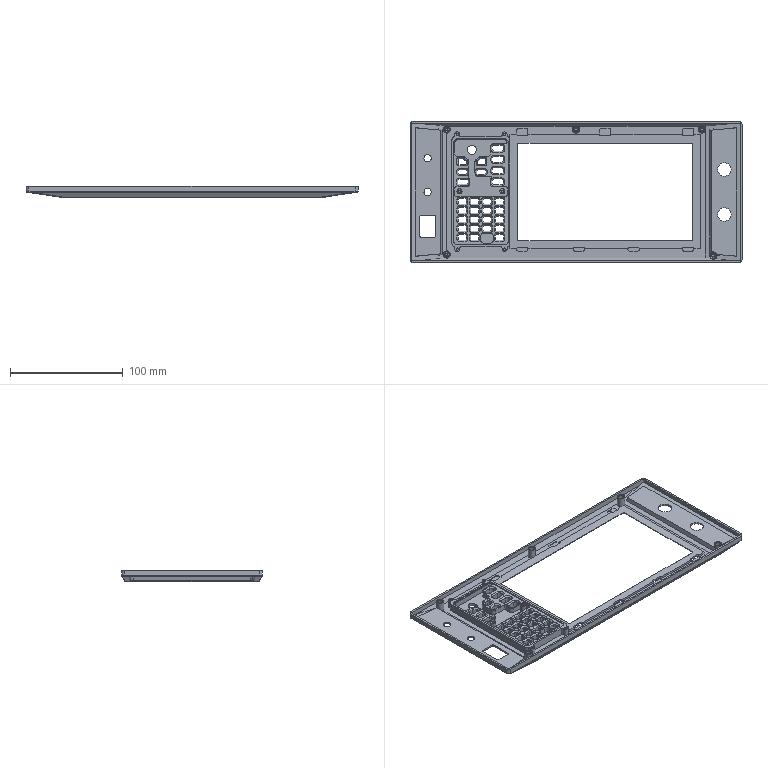NC program | NX | posted with a generic post | part box 295 x 125 x 10 mm
Lines 8754 to 10380 of 10380:
(ZLEVEL_PROFILE_1_COPY_COPY_COPY_COPY_COPY_COPY_COPY , TOOL : D4)
N17464 T04 M6
N17466 G54
N17468 G17 G0 G90 X53.178 Y-46.17 S9500 M3
N17470 G43 Z30. H4
N17472 Z-0.3
N17474 G94 G1 X53.525 Y-46.77 F1000.
N17476 G3 X53.871 Y-46.97 R0.4
N17478 G1 X55.17 F1600.
N17480 Y-45.671
N17482 G3 X54.97 Y-45.325 R0.4
N17484 G1 X54.37 Y-44.978
N17486 G0 X53.178 Y-46.17 Z-0.725
N17488 G1 X53.525 Y-46.77 F1000.
N17490 G3 X53.871 Y-46.97 R0.4
N17492 G1 X55.17 F1600.
N17494 Y-45.671
N17496 G3 X54.97 Y-45.325 R0.4
N17498 G1 X54.37 Y-44.978
N17500 G0 X53.178 Y-46.17 Z-1.15
N17502 G1 X53.525 Y-46.77 F1000.
N17504 G3 X53.871 Y-46.97 R0.4
N17506 G1 X55.17 F1600.
N17508 Y-45.671
N17510 G3 X54.97 Y-45.325 R0.4
N17512 G1 X54.37 Y-44.978
N17514 G0 X53.178 Y-46.17 Z-1.575
N17516 G1 X53.525 Y-46.77 F1000.
N17518 G3 X53.871 Y-46.97 R0.4
N17520 G1 X55.17 F1600.
N17522 Y-45.671
N17524 G3 X54.97 Y-45.325 R0.4
N17526 G1 X54.37 Y-44.978
N17528 G0 X53.178 Y-46.17 Z-2.
N17530 G1 X53.525 Y-46.77 F1000.
N17532 G3 X53.871 Y-46.97 R0.4
N17534 G1 X55.17 F1600.
N17536 Y-45.671
N17538 G3 X54.97 Y-45.325 R0.4
N17540 G1 X54.37 Y-44.978
N17542 G0 Z30.
N17544 Y47.226
N17546 Z-0.3
N17548 G1 X54.97 Y47.572 F1000.
N17550 G3 X55.17 Y47.919 R0.4
N17552 G1 Y48.795 F1600.
N17554 X54.411 Y49.234
N17556 G3 X54.011 Y49.234 R0.4
N17558 G1 X53.411 Y48.887
N17560 G0 Z30.
N17562 X54.37 Y45.958
N17564 Z-0.725
N17566 G1 X54.97 Y46.305 F1000.
N17568 G3 X55.17 Y46.651 R0.4
N17570 G1 Y47.95 F1600.
N17572 X53.871
N17574 G3 X53.525 Y47.75 R0.4
N17576 G1 X53.178 Y47.15
N17578 G0 X54.37 Y45.958 Z-1.15
N17580 G1 X54.97 Y46.305 F1000.
N17582 G3 X55.17 Y46.651 R0.4
N17584 G1 Y47.95 F1600.
N17586 X53.871
N17588 G3 X53.525 Y47.75 R0.4
N17590 G1 X53.178 Y47.15
N17592 G0 X54.37 Y45.958 Z-1.575
N17594 G1 X54.97 Y46.305 F1000.
N17596 G3 X55.17 Y46.651 R0.4
N17598 G1 Y47.95 F1600.
N17600 X53.871
N17602 G3 X53.525 Y47.75 R0.4
N17604 G1 X53.178 Y47.15
N17606 G0 X54.37 Y45.958 Z-2.
N17608 G1 X54.97 Y46.305 F1000.
N17610 G3 X55.17 Y46.651 R0.4
N17612 G1 Y47.95 F1600.
N17614 X53.871
N17616 G3 X53.525 Y47.75 R0.4
N17618 G1 X53.178 Y47.15
N17620 G0 Z30.
N17622 X44.363 Y54.111
N17624 Z-0.3
N17626 G1 Y54.804 F1000.
N17628 G3 X44.163 Y55.15 R0.4
N17630 G1 X43.672 Y55.434 F1600.
N17632 X43.105
N17634 G3 X42.758 Y55.234 R0.4
N17636 G1 X42.412 Y54.634
N17638 G0 Z30.
N17640 X-94.282
N17642 Z-0.3
N17644 G1 X-94.628 Y55.234 F1000.
N17646 G3 X-94.975 Y55.434 R0.4
N17648 G1 X-95.542 F1600.
N17650 X-96.033 Y55.15
N17652 G3 X-96.233 Y54.804 R0.4
N17654 G1 Y54.111
N17656 G0 Z30.
N17658 X-105.281 Y48.887
N17660 Z-0.3
N17662 G1 X-105.881 Y49.233 F1000.
N17664 G3 X-106.281 Y49.233 R0.4
N17666 G1 X-107.04 Y48.795 F1600.
N17668 Y47.919
N17670 G3 X-106.84 Y47.573 R0.4
N17672 G1 X-106.24 Y47.226
N17674 G0 X-105.048 Y47.15 Z-0.725
N17676 G1 X-105.395 Y47.75 F1000.
N17678 G3 X-105.741 Y47.95 R0.4
N17680 G1 X-107.04 F1600.
N17682 Y46.651
N17684 G3 X-106.84 Y46.305 R0.4
N17686 G1 X-106.24 Y45.958
N17688 G0 X-105.048 Y47.15 Z-1.15
N17690 G1 X-105.395 Y47.75 F1000.
N17692 G3 X-105.741 Y47.95 R0.4
N17694 G1 X-107.04 F1600.
N17696 Y46.651
N17698 G3 X-106.84 Y46.305 R0.4
N17700 G1 X-106.24 Y45.958
N17702 G0 X-105.048 Y47.15 Z-1.575
N17704 G1 X-105.395 Y47.75 F1000.
N17706 G3 X-105.741 Y47.95 R0.4
N17708 G1 X-107.04 F1600.
N17710 Y46.651
N17712 G3 X-106.84 Y46.305 R0.4
N17714 G1 X-106.24 Y45.958
N17716 G0 X-105.048 Y47.15 Z-2.
N17718 G1 X-105.395 Y47.75 F1000.
N17720 G3 X-105.741 Y47.95 R0.4
N17722 G1 X-107.04 F1600.
N17724 Y46.651
N17726 G3 X-106.84 Y46.305 R0.4
N17728 G1 X-106.24 Y45.958
N17730 G0 Z30.
N17732 Y-44.978
N17734 Z-0.3
N17736 G1 X-106.84 Y-45.325 F1000.
N17738 G3 X-107.04 Y-45.671 R0.4
N17740 G1 Y-46.97 F1600.
N17742 X-105.741
N17744 G3 X-105.395 Y-46.77 R0.4
N17746 G1 X-105.048 Y-46.17
N17748 G0 X-106.24 Y-44.978 Z-0.725
N17750 G1 X-106.84 Y-45.325 F1000.
N17752 G3 X-107.04 Y-45.671 R0.4
N17754 G1 Y-46.97 F1600.
N17756 X-105.741
N17758 G3 X-105.395 Y-46.77 R0.4
N17760 G1 X-105.048 Y-46.17
N17762 G0 X-106.24 Y-44.978 Z-1.15
N17764 G1 X-106.84 Y-45.325 F1000.
N17766 G3 X-107.04 Y-45.671 R0.4
N17768 G1 Y-46.97 F1600.
N17770 X-105.741
N17772 G3 X-105.395 Y-46.77 R0.4
N17774 G1 X-105.048 Y-46.17
N17776 G0 X-106.24 Y-44.978 Z-1.575
N17778 G1 X-106.84 Y-45.325 F1000.
N17780 G3 X-107.04 Y-45.671 R0.4
N17782 G1 Y-46.97 F1600.
N17784 X-105.741
N17786 G3 X-105.395 Y-46.77 R0.4
N17788 G1 X-105.048 Y-46.17
N17790 G0 X-106.24 Y-44.978 Z-2.
N17792 G1 X-106.84 Y-45.325 F1000.
N17794 G3 X-107.04 Y-45.671 R0.4
N17796 G1 Y-46.97 F1600.
N17798 X-105.741
N17800 G3 X-105.395 Y-46.77 R0.4
N17802 G1 X-105.048 Y-46.17
N17804 G0 Z30.
N17806 M5
(ZLEVEL_PROFILE_1_COPY_COPY_COPY_COPY_COPY_COPY_COPY_COPY , TOOL : D2)
N17808 T02 M6
N17810 G54
N17812 G17 G0 G90 X54.525 Y-47.57 S9500 M3
N17814 G43 Z30. H2
N17816 Z-0.2
N17818 G94 G1 X54.698 Y-47.87 F1000.
N17820 G3 X54.871 Y-47.97 R0.2
N17822 G1 X56.17 F1200.
N17824 Y-46.671
N17826 G3 X56.07 Y-46.498 R0.2
N17828 G1 X55.77 Y-46.325
N17830 G0 X54.525 Y-47.57 Z-0.3
N17832 G1 X54.698 Y-47.87 F1000.
N17834 G3 X54.871 Y-47.97 R0.2
N17836 G1 X56.17 F1200.
N17838 Y-46.671
N17840 G3 X56.07 Y-46.498 R0.2
N17842 G1 X55.77 Y-46.325
N17844 G0 X54.525 Y-47.57 Z-0.5
N17846 G1 X54.698 Y-47.87 F1000.
N17848 G3 X54.871 Y-47.97 R0.2
N17850 G1 X56.17 F1200.
N17852 Y-46.671
N17854 G3 X56.07 Y-46.498 R0.2
N17856 G1 X55.77 Y-46.325
N17858 G0 X54.525 Y-47.57 Z-0.7
N17860 G1 X54.698 Y-47.87 F1000.
N17862 G3 X54.871 Y-47.97 R0.2
N17864 G1 X56.17 F1200.
N17866 Y-46.671
N17868 G3 X56.07 Y-46.498 R0.2
N17870 G1 X55.77 Y-46.325
N17872 G0 X54.525 Y-47.57 Z-0.9
N17874 G1 X54.698 Y-47.87 F1000.
N17876 G3 X54.871 Y-47.97 R0.2
N17878 G1 X56.17 F1200.
N17880 Y-46.671
N17882 G3 X56.07 Y-46.498 R0.2
N17884 G1 X55.77 Y-46.325
N17886 G0 X54.525 Y-47.57 Z-1.1
N17888 G1 X54.698 Y-47.87 F1000.
N17890 G3 X54.871 Y-47.97 R0.2
N17892 G1 X56.17 F1200.
N17894 Y-46.671
N17896 G3 X56.07 Y-46.498 R0.2
N17898 G1 X55.77 Y-46.325
N17900 G0 X54.525 Y-47.57 Z-1.3
N17902 G1 X54.698 Y-47.87 F1000.
N17904 G3 X54.871 Y-47.97 R0.2
N17906 G1 X56.17 F1200.
N17908 Y-46.671
N17910 G3 X56.07 Y-46.498 R0.2
N17912 G1 X55.77 Y-46.325
N17914 G0 X54.525 Y-47.57 Z-1.475
N17916 G1 X54.698 Y-47.87 F1000.
N17918 G3 X54.871 Y-47.97 R0.2
N17920 G1 X56.17 F1200.
N17922 Y-46.671
N17924 G3 X56.07 Y-46.498 R0.2
N17926 G1 X55.77 Y-46.325
N17928 G0 X54.525 Y-47.57 Z-1.65
N17930 G1 X54.698 Y-47.87 F1000.
N17932 G3 X54.871 Y-47.97 R0.2
N17934 G1 X56.17 F1200.
N17936 Y-46.671
N17938 G3 X56.07 Y-46.498 R0.2
N17940 G1 X55.77 Y-46.325
N17942 G0 X54.525 Y-47.57 Z-1.825
N17944 G1 X54.698 Y-47.87 F1000.
N17946 G3 X54.871 Y-47.97 R0.2
N17948 G1 X56.17 F1200.
N17950 Y-46.671
N17952 G3 X56.07 Y-46.498 R0.2
N17954 G1 X55.77 Y-46.325
N17956 G0 X54.525 Y-47.57 Z-2.
N17958 G1 X54.698 Y-47.87 F1000.
N17960 G3 X54.871 Y-47.97 R0.2
N17962 G1 X56.17 F1200.
N17964 Y-46.671
N17966 G3 X56.07 Y-46.498 R0.2
N17968 G1 X55.77 Y-46.325
N17970 G0 Z30.
N17972 Y48.15
N17974 Z-0.2
N17976 G1 X56.07 Y48.323 F1000.
N17978 G3 X56.17 Y48.496 R0.2
N17980 G1 Y49.373 F1200.
N17982 X55.411 Y49.811
N17984 G3 X55.211 Y49.811 R0.2
N17986 G1 X54.911 Y49.638
N17988 G0 X55.77 Y48.15 Z-0.3
N17990 G1 X56.07 Y48.323 F1000.
N17992 G3 X56.17 Y48.496 R0.2
N17994 G1 Y49.373 F1200.
N17996 X55.411 Y49.811
N17998 G3 X55.211 Y49.811 R0.2
N18000 G1 X54.911 Y49.638
N18002 G0 Z30.
N18004 X55.77 Y47.305
N18006 Z-0.5
N18008 G1 X56.07 Y47.478 F1000.
N18010 G3 X56.17 Y47.651 R0.2
N18012 G1 Y48.95 F1200.
N18014 X54.871
N18016 G3 X54.698 Y48.85 R0.2
N18018 G1 X54.525 Y48.55
N18020 G0 X55.77 Y47.305 Z-0.7
N18022 G1 X56.07 Y47.478 F1000.
N18024 G3 X56.17 Y47.651 R0.2
N18026 G1 Y48.95 F1200.
N18028 X54.871
N18030 G3 X54.698 Y48.85 R0.2
N18032 G1 X54.525 Y48.55
N18034 G0 X55.77 Y47.305 Z-0.9
N18036 G1 X56.07 Y47.478 F1000.
N18038 G3 X56.17 Y47.651 R0.2
N18040 G1 Y48.95 F1200.
N18042 X54.871
N18044 G3 X54.698 Y48.85 R0.2
N18046 G1 X54.525 Y48.55
N18048 G0 X55.77 Y47.305 Z-1.1
N18050 G1 X56.07 Y47.478 F1000.
N18052 G3 X56.17 Y47.651 R0.2
N18054 G1 Y48.95 F1200.
N18056 X54.871
N18058 G3 X54.698 Y48.85 R0.2
N18060 G1 X54.525 Y48.55
N18062 G0 X55.77 Y47.305 Z-1.3
N18064 G1 X56.07 Y47.478 F1000.
N18066 G3 X56.17 Y47.651 R0.2
N18068 G1 Y48.95 F1200.
N18070 X54.871
N18072 G3 X54.698 Y48.85 R0.2
N18074 G1 X54.525 Y48.55
N18076 G0 X55.77 Y47.305 Z-1.475
N18078 G1 X56.07 Y47.478 F1000.
N18080 G3 X56.17 Y47.651 R0.2
N18082 G1 Y48.95 F1200.
N18084 X54.871
N18086 G3 X54.698 Y48.85 R0.2
N18088 G1 X54.525 Y48.55
N18090 G0 X55.77 Y47.305 Z-1.65
N18092 G1 X56.07 Y47.478 F1000.
N18094 G3 X56.17 Y47.651 R0.2
N18096 G1 Y48.95 F1200.
N18098 X54.871
N18100 G3 X54.698 Y48.85 R0.2
N18102 G1 X54.525 Y48.55
N18104 G0 X55.77 Y47.305 Z-1.825
N18106 G1 X56.07 Y47.478 F1000.
N18108 G3 X56.17 Y47.651 R0.2
N18110 G1 Y48.95 F1200.
N18112 X54.871
N18114 G3 X54.698 Y48.85 R0.2
N18116 G1 X54.525 Y48.55
N18118 G0 X55.77 Y47.305 Z-2.
N18120 G1 X56.07 Y47.478 F1000.
N18122 G3 X56.17 Y47.651 R0.2
N18124 G1 Y48.95 F1200.
N18126 X54.871
N18128 G3 X54.698 Y48.85 R0.2
N18130 G1 X54.525 Y48.55
N18132 G0 Z30.
N18134 X44.531 Y55.631
N18136 Z-0.2
N18138 G1 Y55.977 F1000.
N18140 G3 X44.431 Y56.15 R0.2
N18142 G1 X43.94 Y56.434 F1200.
N18144 X43.373
N18146 G3 X43.2 Y56.334 R0.2
N18148 G1 X43.026 Y56.034
N18150 G0 X44.531 Y55.631 Z-0.3
N18152 G1 Y55.977 F1000.
N18154 G3 X44.431 Y56.15 R0.2
N18156 G1 X43.94 Y56.434 F1200.
N18158 X43.373
N18160 G3 X43.2 Y56.334 R0.2
N18162 G1 X43.026 Y56.034
N18164 G0 Z30.
N18166 X-94.896
N18168 Z-0.2
N18170 G1 X-95.07 Y56.334 F1000.
N18172 G3 X-95.243 Y56.434 R0.2
N18174 G1 X-95.81 F1200.
N18176 X-96.301 Y56.15
N18178 G3 X-96.401 Y55.977 R0.2
N18180 G1 Y55.631
N18182 G0 X-94.896 Y56.034 Z-0.3
N18184 G1 X-95.07 Y56.334 F1000.
N18186 G3 X-95.243 Y56.434 R0.2
N18188 G1 X-95.81 F1200.
N18190 X-96.301 Y56.15
N18192 G3 X-96.401 Y55.977 R0.2
N18194 G1 Y55.631
N18196 G0 Z30.
N18198 X-106.781 Y49.638
N18200 Z-0.2
N18202 G1 X-107.081 Y49.811 F1000.
N18204 G3 X-107.281 Y49.811 R0.2
N18206 G1 X-108.04 Y49.373 F1200.
N18208 Y48.496
N18210 G3 X-107.94 Y48.323 R0.2
N18212 G1 X-107.64 Y48.15
N18214 G0 X-106.781 Y49.638 Z-0.3
N18216 G1 X-107.081 Y49.811 F1000.
N18218 G3 X-107.281 Y49.811 R0.2
N18220 G1 X-108.04 Y49.373 F1200.
N18222 Y48.496
N18224 G3 X-107.94 Y48.323 R0.2
N18226 G1 X-107.64 Y48.15
N18228 G0 X-106.395 Y48.55 Z-0.5
N18230 G1 X-106.568 Y48.85 F1000.
N18232 G3 X-106.741 Y48.95 R0.2
N18234 G1 X-108.04 F1200.
N18236 Y47.651
N18238 G3 X-107.94 Y47.478 R0.2
N18240 G1 X-107.64 Y47.305
N18242 G0 X-106.395 Y48.55 Z-0.7
N18244 G1 X-106.568 Y48.85 F1000.
N18246 G3 X-106.741 Y48.95 R0.2
N18248 G1 X-108.04 F1200.
N18250 Y47.651
N18252 G3 X-107.94 Y47.478 R0.2
N18254 G1 X-107.64 Y47.305
N18256 G0 X-106.395 Y48.55 Z-0.9
N18258 G1 X-106.568 Y48.85 F1000.
N18260 G3 X-106.741 Y48.95 R0.2
N18262 G1 X-108.04 F1200.
N18264 Y47.651
N18266 G3 X-107.94 Y47.478 R0.2
N18268 G1 X-107.64 Y47.305
N18270 G0 X-106.395 Y48.55 Z-1.1
N18272 G1 X-106.568 Y48.85 F1000.
N18274 G3 X-106.741 Y48.95 R0.2
N18276 G1 X-108.04 F1200.
N18278 Y47.651
N18280 G3 X-107.94 Y47.478 R0.2
N18282 G1 X-107.64 Y47.305
N18284 G0 X-106.395 Y48.55 Z-1.3
N18286 G1 X-106.568 Y48.85 F1000.
N18288 G3 X-106.741 Y48.95 R0.2
N18290 G1 X-108.04 F1200.
N18292 Y47.651
N18294 G3 X-107.94 Y47.478 R0.2
N18296 G1 X-107.64 Y47.305
N18298 G0 X-106.395 Y48.55 Z-1.475
N18300 G1 X-106.568 Y48.85 F1000.
N18302 G3 X-106.741 Y48.95 R0.2
N18304 G1 X-108.04 F1200.
N18306 Y47.651
N18308 G3 X-107.94 Y47.478 R0.2
N18310 G1 X-107.64 Y47.305
N18312 G0 X-106.395 Y48.55 Z-1.65
N18314 G1 X-106.568 Y48.85 F1000.
N18316 G3 X-106.741 Y48.95 R0.2
N18318 G1 X-108.04 F1200.
N18320 Y47.651
N18322 G3 X-107.94 Y47.478 R0.2
N18324 G1 X-107.64 Y47.305
N18326 G0 X-106.395 Y48.55 Z-1.825
N18328 G1 X-106.568 Y48.85 F1000.
N18330 G3 X-106.741 Y48.95 R0.2
N18332 G1 X-108.04 F1200.
N18334 Y47.651
N18336 G3 X-107.94 Y47.478 R0.2
N18338 G1 X-107.64 Y47.305
N18340 G0 X-106.395 Y48.55 Z-2.
N18342 G1 X-106.568 Y48.85 F1000.
N18344 G3 X-106.741 Y48.95 R0.2
N18346 G1 X-108.04 F1200.
N18348 Y47.651
N18350 G3 X-107.94 Y47.478 R0.2
N18352 G1 X-107.64 Y47.305
N18354 G0 Z30.
N18356 Y-46.325
N18358 Z-0.2
N18360 G1 X-107.94 Y-46.498 F1000.
N18362 G3 X-108.04 Y-46.671 R0.2
N18364 G1 Y-47.97 F1200.
N18366 X-106.741
N18368 G3 X-106.568 Y-47.87 R0.2
N18370 G1 X-106.395 Y-47.57
N18372 G0 X-107.64 Y-46.325 Z-0.3
N18374 G1 X-107.94 Y-46.498 F1000.
N18376 G3 X-108.04 Y-46.671 R0.2
N18378 G1 Y-47.97 F1200.
N18380 X-106.741
N18382 G3 X-106.568 Y-47.87 R0.2
N18384 G1 X-106.395 Y-47.57
N18386 G0 X-107.64 Y-46.325 Z-0.5
N18388 G1 X-107.94 Y-46.498 F1000.
N18390 G3 X-108.04 Y-46.671 R0.2
N18392 G1 Y-47.97 F1200.
N18394 X-106.741
N18396 G3 X-106.568 Y-47.87 R0.2
N18398 G1 X-106.395 Y-47.57
N18400 G0 X-107.64 Y-46.325 Z-0.7
N18402 G1 X-107.94 Y-46.498 F1000.
N18404 G3 X-108.04 Y-46.671 R0.2
N18406 G1 Y-47.97 F1200.
N18408 X-106.741
N18410 G3 X-106.568 Y-47.87 R0.2
N18412 G1 X-106.395 Y-47.57
N18414 G0 X-107.64 Y-46.325 Z-0.9
N18416 G1 X-107.94 Y-46.498 F1000.
N18418 G3 X-108.04 Y-46.671 R0.2
N18420 G1 Y-47.97 F1200.
N18422 X-106.741
N18424 G3 X-106.568 Y-47.87 R0.2
N18426 G1 X-106.395 Y-47.57
N18428 G0 X-107.64 Y-46.325 Z-1.1
N18430 G1 X-107.94 Y-46.498 F1000.
N18432 G3 X-108.04 Y-46.671 R0.2
N18434 G1 Y-47.97 F1200.
N18436 X-106.741
N18438 G3 X-106.568 Y-47.87 R0.2
N18440 G1 X-106.395 Y-47.57
N18442 G0 X-107.64 Y-46.325 Z-1.3
N18444 G1 X-107.94 Y-46.498 F1000.
N18446 G3 X-108.04 Y-46.671 R0.2
N18448 G1 Y-47.97 F1200.
N18450 X-106.741
N18452 G3 X-106.568 Y-47.87 R0.2
N18454 G1 X-106.395 Y-47.57
N18456 G0 X-107.64 Y-46.325 Z-1.475
N18458 G1 X-107.94 Y-46.498 F1000.
N18460 G3 X-108.04 Y-46.671 R0.2
N18462 G1 Y-47.97 F1200.
N18464 X-106.741
N18466 G3 X-106.568 Y-47.87 R0.2
N18468 G1 X-106.395 Y-47.57
N18470 G0 X-107.64 Y-46.325 Z-1.65
N18472 G1 X-107.94 Y-46.498 F1000.
N18474 G3 X-108.04 Y-46.671 R0.2
N18476 G1 X-108.039 Y-47.97 F1200.
N18478 X-106.741
N18480 G3 X-106.568 Y-47.87 R0.2
N18482 G1 X-106.395 Y-47.57
N18484 G0 X-107.64 Y-46.325 Z-1.825
N18486 G1 X-107.94 Y-46.498 F1000.
N18488 G3 X-108.04 Y-46.671 R0.2
N18490 G1 X-108.039 Y-47.97 F1200.
N18492 X-106.741
N18494 G3 X-106.568 Y-47.87 R0.2
N18496 G1 X-106.395 Y-47.57
N18498 G0 X-107.64 Y-46.325 Z-2.
N18500 G1 X-107.94 Y-46.498 F1000.
N18502 G3 X-108.04 Y-46.671 R0.2
N18504 G1 X-108.039 Y-47.97 F1200.
N18506 X-106.741
N18508 G3 X-106.568 Y-47.87 R0.2
N18510 G1 X-106.395 Y-47.57
N18512 G0 Z30.
N18514 M5
(ZLEVEL_PROFILE_1_COPY_COPY_COPY_COPY_COPY , TOOL : D2R0.5)
N18516 T05 M6
N18518 G54
N18520 G17 G0 G90 X51.029 Y45.352 S9500 M3
N18522 G43 Z30. H5
N18524 Z-0.532
N18526 G94 G1 Z-2.032 F1000.
N18528 X50.843 Y45.674
N18530 G3 X50.67 Y45.774 R0.2
N18532 G1 X-102.54 F3000.
N18534 G3 X-105.864 Y42.45 R3.324
N18536 G1 Y-42.47
N18538 G3 X-102.54 Y-45.794 R3.324
N18540 G1 X50.67
N18542 G3 X53.994 Y-42.47 R3.324
N18544 G1 Y42.45
N18546 G3 X50.67 Y45.774 R3.324
N18548 G1 Y45.679 Z-2.063
N18550 G2 X53.899 Y42.45 R3.229
N18552 G1 Y-42.47
N18554 G2 X50.67 Y-45.699 R3.229
N18556 G1 X-102.54
N18558 G2 X-105.769 Y-42.47 R3.229
N18560 G1 Y42.45
N18562 G2 X-102.54 Y45.679 R3.229
N18564 G1 X50.67
N18566 Y45.584 Z-2.095
N18568 X-102.54
N18570 G3 X-105.674 Y42.45 R3.134
N18572 G1 Y-42.47
N18574 G3 X-102.54 Y-45.604 R3.134
N18576 G1 X50.67
N18578 G3 X53.804 Y-42.47 R3.134
N18580 G1 Y42.45
N18582 G3 X50.67 Y45.584 R3.134
N18584 G1 Y45.489 Z-2.126
N18586 G2 X53.709 Y42.45 R3.039
N18588 G1 Y-42.47
N18590 G2 X50.67 Y-45.509 R3.039
N18592 G1 X-102.54
N18594 G2 X-105.579 Y-42.47 R3.039
N18596 G1 Y42.45
N18598 G2 X-102.54 Y45.489 R3.039
N18600 G1 X50.67
N18602 Y45.395 Z-2.158
N18604 X-102.54
N18606 G3 X-105.485 Y42.45 R2.945
N18608 G1 Y-42.47
N18610 G3 X-102.54 Y-45.415 R2.945
N18612 G1 X50.67
N18614 G3 X53.615 Y-42.47 R2.945
N18616 G1 Y42.45
N18618 G3 X50.67 Y45.395 R2.945
N18620 G1 Y45.3 Z-2.19
N18622 G2 X53.52 Y42.45 R2.85
N18624 G1 Y-42.47
N18626 G2 X50.67 Y-45.32 R2.85
N18628 G1 X-102.54
N18630 G2 X-105.39 Y-42.47 R2.85
N18632 G1 Y42.45
N18634 G2 X-102.54 Y45.3 R2.85
N18636 G1 X50.67
N18638 Y45.205 Z-2.221
N18640 X-102.54
N18642 G3 X-105.295 Y42.45 R2.755
N18644 G1 Y-42.47
N18646 G3 X-102.54 Y-45.225 R2.755
N18648 G1 X50.67
N18650 G3 X53.425 Y-42.47 R2.755
N18652 G1 Y42.45
N18654 G3 X50.67 Y45.205 R2.755
N18656 G1 Y45.11 Z-2.253
N18658 G2 X53.33 Y42.45 R2.66
N18660 G1 Y-42.47
N18662 G2 X50.67 Y-45.13 R2.66
N18664 G1 X-102.54
N18666 G2 X-105.2 Y-42.47 R2.66
N18668 G1 Y42.45
N18670 G2 X-102.54 Y45.11 R2.66
N18672 G1 X50.67
N18674 Y45.015 Z-2.285
N18676 X-102.54
N18678 G3 X-105.105 Y42.45 R2.565
N18680 G1 Y-42.47
N18682 G3 X-102.54 Y-45.035 R2.565
N18684 G1 X50.67
N18686 G3 X53.235 Y-42.47 R2.565
N18688 G1 Y42.45
N18690 G3 X50.67 Y45.015 R2.565
N18692 G1 Y44.92 Z-2.316
N18694 G2 X53.14 Y42.45 R2.47
N18696 G1 Y-42.47
N18698 G2 X50.67 Y-44.94 R2.47
N18700 G1 X-102.54
N18702 G2 X-105.01 Y-42.47 R2.47
N18704 G1 Y42.45
N18706 G2 X-102.54 Y44.92 R2.47
N18708 G1 X50.67
N18710 Y44.825 Z-2.348
N18712 X-102.54
N18714 G3 X-104.915 Y42.45 R2.375
N18716 G1 Y-42.47
N18718 G3 X-102.54 Y-44.845 R2.375
N18720 G1 X50.67
N18722 G3 X53.045 Y-42.47 R2.375
N18724 G1 Y42.45
N18726 G3 X50.67 Y44.825 R2.375
N18728 G1 Y44.73 Z-2.379
N18730 G2 X52.95 Y42.45 R2.28
N18732 G1 Y-42.47
N18734 G2 X50.67 Y-44.75 R2.28
N18736 G1 X-102.54
N18738 G2 X-104.82 Y-42.47 R2.28
N18740 G1 Y42.45
N18742 G2 X-102.54 Y44.73 R2.28
N18744 G1 X50.67
N18746 Y44.636 Z-2.411
N18748 X-102.54
N18750 G3 X-104.726 Y42.45 R2.186
N18752 G1 Y-42.47
N18754 G3 X-102.54 Y-44.656 R2.186
N18756 G1 X50.67
N18758 G3 X52.856 Y-42.47 R2.186
N18760 G1 Y42.45
N18762 G3 X50.67 Y44.636 R2.186
N18764 G1 Y44.541 Z-2.443
N18766 G2 X52.761 Y42.45 R2.091
N18768 G1 Y-42.47
N18770 G2 X50.67 Y-44.561 R2.091
N18772 G1 X-102.54
N18774 G2 X-104.631 Y-42.47 R2.091
N18776 G1 Y42.45
N18778 G2 X-102.54 Y44.541 R2.091
N18780 G1 X50.67
N18782 Y44.446 Z-2.474
N18784 X-102.54
N18786 G3 X-104.536 Y42.45 R1.996
N18788 G1 Y-42.47
N18790 G3 X-102.54 Y-44.466 R1.996
N18792 G1 X50.67
N18794 G3 X52.666 Y-42.47 R1.996
N18796 G1 Y42.45
N18798 G3 X50.67 Y44.446 R1.996
N18800 G1 Y44.351 Z-2.506
N18802 G2 X52.571 Y42.45 R1.901
N18804 G1 Y-42.47
N18806 G2 X50.67 Y-44.371 R1.901
N18808 G1 X-102.54
N18810 G2 X-104.441 Y-42.47 R1.901
N18812 G1 Y42.45
N18814 G2 X-102.54 Y44.351 R1.901
N18816 G1 X50.67
N18818 Y44.256 Z-2.538
N18820 X-102.54
N18822 G3 X-104.346 Y42.45 R1.806
N18824 G1 Y-42.47
N18826 G3 X-102.54 Y-44.276 R1.806
N18828 G1 X50.67
N18830 G3 X52.476 Y-42.47 R1.806
N18832 G1 Y42.45
N18834 G3 X50.67 Y44.256 R1.806
N18836 G1 Y44.161 Z-2.569
N18838 G2 X52.381 Y42.45 R1.711
N18840 G1 Y-42.47
N18842 G2 X50.67 Y-44.181 R1.711
N18844 G1 X-102.54
N18846 G2 X-104.251 Y-42.47 R1.711
N18848 G1 Y42.45
N18850 G2 X-102.54 Y44.161 R1.711
N18852 G1 X50.67
N18854 Y44.066 Z-2.601
N18856 X-102.54
N18858 G3 X-104.156 Y42.45 R1.616
N18860 G1 Y-42.47
N18862 G3 X-102.54 Y-44.086 R1.616
N18864 G1 X50.67
N18866 G3 X52.286 Y-42.47 R1.616
N18868 G1 Y42.45
N18870 G3 X50.67 Y44.066 R1.616
N18872 G1 Y43.971 Z-2.632
N18874 G2 X52.191 Y42.45 R1.521
N18876 G1 Y-42.47
N18878 G2 X50.67 Y-43.991 R1.521
N18880 G1 X-102.54
N18882 G2 X-104.061 Y-42.47 R1.521
N18884 G1 Y42.45
N18886 G2 X-102.54 Y43.971 R1.521
N18888 G1 X50.67
N18890 Y43.877 Z-2.664
N18892 X-102.54
N18894 G3 X-103.967 Y42.45 R1.427
N18896 G1 Y-42.47
N18898 G3 X-102.54 Y-43.897 R1.427
N18900 G1 X50.67
N18902 G3 X52.097 Y-42.47 R1.427
N18904 G1 Y42.45
N18906 G3 X50.67 Y43.877 R1.427
N18908 G1 Y43.782 Z-2.696
N18910 G2 X52.002 Y42.45 R1.332
N18912 G1 Y-42.47
N18914 G2 X50.67 Y-43.802 R1.332
N18916 G1 X-102.54
N18918 G2 X-103.872 Y-42.47 R1.332
N18920 G1 Y42.45
N18922 G2 X-102.54 Y43.782 R1.332
N18924 G1 X50.67
N18926 Y43.687 Z-2.727
N18928 X-102.54
N18930 G3 X-103.777 Y42.45 R1.237
N18932 G1 Y-42.47
N18934 G3 X-102.54 Y-43.707 R1.237
N18936 G1 X50.67
N18938 G3 X51.907 Y-42.47 R1.237
N18940 G1 Y42.45
N18942 G3 X50.67 Y43.687 R1.237
N18944 G1 Y43.592 Z-2.759
N18946 G2 X51.812 Y42.45 R1.142
N18948 G1 Y-42.47
N18950 G2 X50.67 Y-43.612 R1.142
N18952 G1 X-102.54
N18954 G2 X-103.682 Y-42.47 R1.142
N18956 G1 Y42.45
N18958 G2 X-102.54 Y43.592 R1.142
N18960 G1 X50.67
N18962 Y43.497 Z-2.791
N18964 X-102.54
N18966 G3 X-103.587 Y42.45 R1.047
N18968 G1 Y-42.47
N18970 G3 X-102.54 Y-43.517 R1.047
N18972 G1 X50.67
N18974 G3 X51.717 Y-42.47 R1.047
N18976 G1 Y42.45
N18978 G3 X50.67 Y43.497 R1.047
N18980 G1 Y43.402 Z-2.822
N18982 G2 X51.622 Y42.45 R0.952
N18984 G1 Y-42.47
N18986 G2 X50.67 Y-43.422 R0.952
N18988 G1 X-102.54
N18990 G2 X-103.492 Y-42.47 R0.952
N18992 G1 Y42.45
N18994 G2 X-102.54 Y43.402 R0.952
N18996 G1 X50.67
N18998 Y43.307 Z-2.854
N19000 X-102.54
N19002 G3 X-103.397 Y42.45 R0.857
N19004 G1 Y-42.47
N19006 G3 X-102.54 Y-43.327 R0.857
N19008 G1 X50.67
N19010 G3 X51.527 Y-42.47 R0.857
N19012 G1 Y42.45
N19014 G3 X50.67 Y43.307 R0.857
N19016 G1 Y43.213 Z-2.885
N19018 G2 X51.433 Y42.45 R0.763
N19020 G1 Y-42.47
N19022 G2 X50.67 Y-43.233 R0.763
N19024 G1 X-102.54
N19026 G2 X-103.303 Y-42.47 R0.763
N19028 G1 Y42.45
N19030 G2 X-102.54 Y43.213 R0.763
N19032 G1 X50.67
N19034 Y43.118 Z-2.917
N19036 X-102.54
N19038 G3 X-103.208 Y42.45 R0.668
N19040 G1 Y-42.47
N19042 G3 X-102.54 Y-43.138 R0.668
N19044 G1 X50.67
N19046 G3 X51.338 Y-42.47 R0.668
N19048 G1 Y42.45
N19050 G3 X50.67 Y43.118 R0.668
N19052 G1 Y43.023 Z-2.949
N19054 G2 X51.243 Y42.45 R0.573
N19056 G1 Y-42.47
N19058 G2 X50.67 Y-43.043 R0.573
N19060 G1 X-102.54
N19062 G2 X-103.113 Y-42.47 R0.573
N19064 G1 Y42.45
N19066 G2 X-102.54 Y43.023 R0.573
N19068 G1 X50.67
N19070 Y42.928 Z-2.98
N19072 X-102.54
N19074 G3 X-103.018 Y42.45 R0.478
N19076 G1 Y-42.47
N19078 G3 X-102.54 Y-42.948 R0.478
N19080 G1 X50.67
N19082 G3 X51.148 Y-42.47 R0.478
N19084 G1 Y42.45
N19086 G3 X50.67 Y42.928 R0.478
N19088 G1 Y42.833 Z-3.012
N19090 G2 X51.053 Y42.45 R0.383
N19092 G1 Y-42.47
N19094 G2 X50.67 Y-42.853 R0.383
N19096 G1 X-102.54
N19098 G2 X-102.923 Y-42.47 R0.383
N19100 G1 Y42.45
N19102 G2 X-102.54 Y42.833 R0.383
N19104 G1 X50.67
N19106 X50.669 Y42.785 Z-3.028
N19108 X50.668 Y42.738 Z-3.044
N19110 X-102.534
N19112 G3 X-102.828 Y42.444 R0.294
N19114 G1 Y-42.464
N19116 G3 X-102.534 Y-42.758 R0.294
N19118 G1 X50.664
N19120 G3 X50.958 Y-42.464 R0.294
N19122 G1 Y42.444
N19124 G3 X50.668 Y42.738 R0.294
N19126 G1 X50.666 Y42.689 Z-3.059
N19128 X50.664 Y42.642 Z-3.075
N19130 G2 X50.863 Y42.434 R0.208
N19132 G1 Y-42.455
N19134 G2 X50.655 Y-42.663 R0.208
N19136 G1 X-102.525
N19138 G2 X-102.733 Y-42.455 R0.208
N19140 G1 Y42.435
N19142 G2 X-102.525 Y42.643 R0.208
N19144 G1 X50.664 Y42.642
N19146 X50.663 Y42.594 Z-3.091
N19148 X50.661 Y42.547 Z-3.107
N19150 X-102.528
N19152 X-102.588 Y42.542
N19154 X-102.631 Y42.498
N19156 X-102.637 Y42.439
N19158 Y-42.442
N19160 X-102.547 Y-42.565
N19162 X50.658 Y-42.567
N19164 X50.718 Y-42.562
N19166 X50.761 Y-42.518
N19168 X50.767 Y-42.459
N19170 Y42.438
N19172 X50.762 Y42.497
N19174 X50.72 Y42.54
N19176 X50.661 Y42.547
N19178 X50.658 Y42.498 Z-3.123
N19180 X50.655 Y42.45 Z-3.138
N19182 Y-42.47
N19184 X-102.447 Y-42.472
N19186 X-102.54 Y-42.442
N19188 X-102.525 Y42.45
N19190 X50.655
N19192 G2 X50.555 Y42.277 R0.2
N19194 G1 X50.163 Y42.05
N19196 Z-1.638
N19198 G0 Z30.
N19200 X50.084 Y41.957
N19202 Z-1.67
N19204 G1 Z-3.17 F1000.
N19206 X50.477 Y42.184
N19208 G3 X50.577 Y42.357 R0.2
N19210 G1 X-102.447 Y42.358 F3000.
N19212 X-102.448 Y-42.375
N19214 X50.577 Y-42.378
N19216 Y42.357
N19218 G3 X50.404 Y42.257 R0.2
N19220 G1 X50.177 Y41.865
N19222 Z-1.67
N19224 G0 Z30.
N19226 M5
(ZLEVEL_PROFILE_COPY_1 , TOOL : D6A45)
N19228 T07 M6
N19230 G54
N19232 G17 G0 G90 X72.81 Y30.012 S9500 M3
N19234 G43 Z30. H7
N19236 Z0.5
N19238 G94 G1 Z-1. F1000.
N19240 X73.02 Y30.391
N19242 G3 X72.5 Y30.691 R0.6
N19244 G1 X66.5
N19246 G3 X65.259 Y29.45 R1.241
N19248 G1 Y28.45
N19250 G3 X66.5 Y27.209 R1.241
N19252 G1 X72.5
N19254 G3 X73.741 Y28.45 R1.241
N19256 G1 Y29.45
N19258 G3 X72.5 Y30.691 R1.241
N19260 X71.98 Y30.391 R0.6
N19262 G1 X71.807 Y30.091
N19264 Z0.5
N19266 G0 Z30.
N19268 X98.859 Y25.901
N19270 Z0.5
N19272 G1 Z-1.
N19274 X98.559 Y25.728
N19276 G3 X98.259 Y25.209 R0.6
N19278 G1 X103.741
N19280 Y28.691
N19282 X101.077
N19284 G2 X98.259 Y26.628 R12.259
N19286 G1 Y25.209
N19288 G3 X98.778 Y25.509 R0.6
N19290 G1 X98.951 Y25.809
N19292 Z0.5
N19294 G0 Z30.
N19296 X81.859 Y25.901
N19298 Z0.5
N19300 G1 Z-1.
N19302 X81.559 Y25.728
N19304 G3 X81.259 Y25.209 R0.6
N19306 G1 X86.741
N19308 Y26.628
N19310 G2 X83.923 Y28.691 R12.259
N19312 G1 X81.259
N19314 Y25.209
N19316 G3 X81.778 Y25.509 R0.6
N19318 G1 X81.951 Y25.809
N19320 Z0.5
N19322 G0 Z30.
N19324 X72.81 Y20.012
N19326 Z0.5
N19328 G1 Z-1.
N19330 X73.02 Y20.391
N19332 G3 X72.5 Y20.691 R0.6
N19334 G1 X66.5
N19336 G3 X65.259 Y19.45 R1.241
N19338 G1 Y18.45
N19340 G3 X66.5 Y17.209 R1.241
N19342 G1 X72.5
N19344 G3 X73.741 Y18.45 R1.241
N19346 G1 Y19.45
N19348 G3 X72.5 Y20.691 R1.241
N19350 X71.98 Y20.391 R0.6
N19352 G1 X71.807 Y20.091
N19354 Z0.5
N19356 G0 Z30.
N19358 X103.31 Y18.262
N19360 Z0.5
N19362 G1 Z-1.
N19364 X103.52 Y18.641
N19366 G3 X103. Y18.941 R0.6
N19368 G1 X98.
N19370 G3 X97.759 Y18.7 R0.241
N19372 G1 Y16.7
N19374 G3 X98. Y16.459 R0.241
N19376 G1 X103.
N19378 G3 X104.241 Y17.7 R1.241
N19380 X103. Y18.941 R1.241
N19382 X102.48 Y18.641 R0.6
N19384 G1 X102.307 Y18.341
N19386 Z0.5
N19388 G0 Z30.
N19390 X86.561
N19392 Z0.5
N19394 G1 Z-1.
N19396 X86.7 Y18.422
N19398 G3 X87. Y18.941 R0.6
N19400 G1 X82.
N19402 G3 X80.759 Y17.7 R1.241
N19404 X82. Y16.459 R1.241
N19406 G1 X87.
N19408 G3 X87.241 Y16.7 R0.241
N19410 G1 Y18.7
N19412 G3 X87. Y18.941 R0.241
N19414 X86.48 Y18.641 R0.6
N19416 G1 X86.307 Y18.341
N19418 Z0.5
N19420 G0 Z30.
N19422 X103.561 Y9.591
N19424 Z0.5
N19426 G1 Z-1.
N19428 X103.7 Y9.672
N19430 G3 X104. Y10.191 R0.6
N19432 G1 X97.
N19434 G3 X96.759 Y9.95 R0.241
N19436 G1 Y7.95
N19438 G3 X97. Y7.709 R0.241
N19440 G1 X104.
N19442 G3 X104.241 Y7.95 R0.241
N19444 G1 Y9.95
N19446 G3 X104. Y10.191 R0.241
N19448 X103.48 Y9.891 R0.6
N19450 G1 X103.307 Y9.591
N19452 Z0.5
N19454 G0 Z30.
N19456 X72.81 Y10.012
N19458 Z0.5
N19460 G1 Z-1.
N19462 X73.02 Y10.391
N19464 G3 X72.5 Y10.691 R0.6
N19466 G1 X66.5
N19468 G3 X65.259 Y9.45 R1.241
N19470 G1 Y8.45
N19472 G3 X66.5 Y7.209 R1.241
N19474 G1 X72.5
N19476 G3 X73.741 Y8.45 R1.241
N19478 G1 Y9.45
N19480 G3 X72.5 Y10.691 R1.241
N19482 X71.98 Y10.391 R0.6
N19484 G1 X71.807 Y10.091
N19486 Z0.5
N19488 G0 Z30.
N19490 X103.019 Y-7.129
N19492 Z0.5
N19494 G1 Z-1.
N19496 X103.114 Y-7.066
N19498 G3 X103.382 Y-6.529 R0.6
N19500 G1 X98.618
N19502 G3 X98.402 Y-6.662 R0.241
N19504 G1 X98.284 Y-6.898
N19506 X98.255 Y-6.948
N19508 X98.259 Y-7.006
N19510 Y-9.534
N19512 X98.255 Y-9.592
N19514 X98.284 Y-9.642
N19516 X98.402 Y-9.878
N19518 G3 X98.618 Y-10.011 R0.241
N19520 G1 X103.382
N19522 G3 X103.598 Y-9.878 R0.241
N19524 G1 X103.716 Y-9.642
N19526 X103.745 Y-9.592
N19528 X103.741 Y-9.534
N19530 Y-7.006
N19532 X103.745 Y-6.948
N19534 X103.716 Y-6.898
N19536 X103.598 Y-6.662
N19538 G3 X103.382 Y-6.529 R0.241
N19540 X102.862 Y-6.829 R0.6
N19542 G1 X102.689 Y-7.129
N19544 Z0.5
N19546 G0 Z30.
N19548 X87.981 Y-9.411
N19550 Z0.5
N19552 G1 Z-1.
N19554 X87.886 Y-9.474
N19556 G3 X87.618 Y-10.011 R0.6
N19558 G1 X92.382
N19560 G3 X92.598 Y-9.878 R0.241
N19562 G1 X92.716 Y-9.642
N19564 X92.745 Y-9.592
N19566 X92.741 Y-9.534
N19568 Y-7.006
N19570 X92.745 Y-6.948
N19572 X92.716 Y-6.898
N19574 X92.598 Y-6.662
N19576 G3 X92.382 Y-6.529 R0.241
N19578 G1 X87.618
N19580 G3 X87.402 Y-6.662 R0.241
N19582 G1 X87.284 Y-6.898
N19584 X87.255 Y-6.948
N19586 X87.259 Y-7.006
N19588 Y-9.534
N19590 X87.255 Y-9.592
N19592 X87.284 Y-9.642
N19594 X87.402 Y-9.878
N19596 G3 X87.618 Y-10.011 R0.241
N19598 X88.138 Y-9.711 R0.6
N19600 G1 X88.311 Y-9.411
N19602 Z0.5
N19604 G0 Z30.
N19606 X76.981
N19608 Z0.5
N19610 G1 Z-1.
N19612 X76.886 Y-9.474
N19614 G3 X76.618 Y-10.011 R0.6
N19616 G1 X81.382
N19618 G3 X81.598 Y-9.878 R0.241
N19620 G1 X81.716 Y-9.642
N19622 X81.745 Y-9.592
N19624 X81.741 Y-9.534
N19626 Y-7.006
N19628 X81.745 Y-6.948
N19630 X81.716 Y-6.898
N19632 X81.598 Y-6.662
N19634 G3 X81.382 Y-6.529 R0.241
N19636 G1 X76.618
N19638 G3 X76.402 Y-6.662 R0.241
N19640 G1 X76.284 Y-6.898
N19642 X76.255 Y-6.948
N19644 X76.259 Y-7.006
N19646 Y-9.534
N19648 X76.255 Y-9.592
N19650 X76.284 Y-9.642
N19652 X76.402 Y-9.878
N19654 G3 X76.618 Y-10.011 R0.241
N19656 X77.138 Y-9.711 R0.6
N19658 G1 X77.311 Y-9.411
N19660 Z0.5
N19662 G0 Z30.
N19664 X65.981
N19666 Z0.5
N19668 G1 Z-1.
N19670 X65.886 Y-9.474
N19672 G3 X65.618 Y-10.011 R0.6
N19674 G1 X70.382
N19676 G3 X70.598 Y-9.878 R0.241
N19678 G1 X70.716 Y-9.642
N19680 X70.745 Y-9.592
N19682 X70.741 Y-9.534
N19684 Y-7.006
N19686 X70.745 Y-6.948
N19688 X70.716 Y-6.898
N19690 X70.598 Y-6.662
N19692 G3 X70.382 Y-6.529 R0.241
N19694 G1 X65.618
N19696 G3 X65.402 Y-6.662 R0.241
N19698 G1 X65.284 Y-6.898
N19700 X65.255 Y-6.948
N19702 X65.259 Y-7.006
N19704 Y-9.534
N19706 X65.255 Y-9.592
N19708 X65.284 Y-9.642
N19710 X65.402 Y-9.878
N19712 G3 X65.618 Y-10.011 R0.241
N19714 X66.138 Y-9.711 R0.6
N19716 G1 X66.311 Y-9.411
N19718 Z0.5
N19720 G0 Z30.
N19722 X98.981 Y-17.411
N19724 Z0.5
N19726 G1 Z-1.
N19728 X98.886 Y-17.474
N19730 G3 X98.618 Y-18.011 R0.6
N19732 G1 X103.382
N19734 G3 X103.598 Y-17.878 R0.241
N19736 G1 X103.716 Y-17.642
N19738 X103.745 Y-17.592
N19740 X103.741 Y-17.534
N19742 Y-15.006
N19744 X103.745 Y-14.948
N19746 X103.716 Y-14.898
N19748 X103.598 Y-14.662
N19750 G3 X103.382 Y-14.529 R0.241
N19752 G1 X98.618
N19754 G3 X98.402 Y-14.662 R0.241
N19756 G1 X98.284 Y-14.898
N19758 X98.255 Y-14.948
N19760 X98.259 Y-15.006
N19762 Y-17.534
N19764 X98.255 Y-17.592
N19766 X98.284 Y-17.642
N19768 X98.402 Y-17.878
N19770 G3 X98.618 Y-18.011 R0.241
N19772 X99.138 Y-17.711 R0.6
N19774 G1 X99.311 Y-17.411
N19776 Z0.5
N19778 G0 Z30.
N19780 X87.981
N19782 Z0.5
N19784 G1 Z-1.
N19786 X87.886 Y-17.474
N19788 G3 X87.618 Y-18.011 R0.6
N19790 G1 X92.382
N19792 G3 X92.598 Y-17.878 R0.241
N19794 G1 X92.716 Y-17.642
N19796 X92.745 Y-17.592
N19798 X92.741 Y-17.534
N19800 Y-15.006
N19802 X92.745 Y-14.948
N19804 X92.716 Y-14.898
N19806 X92.598 Y-14.662
N19808 G3 X92.382 Y-14.529 R0.241
N19810 G1 X87.618
N19812 G3 X87.402 Y-14.662 R0.241
N19814 G1 X87.284 Y-14.898
N19816 X87.255 Y-14.948
N19818 X87.259 Y-15.006
N19820 Y-17.534
N19822 X87.255 Y-17.592
N19824 X87.284 Y-17.642
N19826 X87.402 Y-17.878
N19828 G3 X87.618 Y-18.011 R0.241
N19830 X88.138 Y-17.711 R0.6
N19832 G1 X88.311 Y-17.411
N19834 Z0.5
N19836 G0 Z30.
N19838 X76.981
N19840 Z0.5
N19842 G1 Z-1.
N19844 X76.886 Y-17.474
N19846 G3 X76.618 Y-18.011 R0.6
N19848 G1 X81.382
N19850 G3 X81.598 Y-17.878 R0.241
N19852 G1 X81.716 Y-17.642
N19854 X81.745 Y-17.592
N19856 X81.741 Y-17.534
N19858 Y-15.006
N19860 X81.745 Y-14.948
N19862 X81.716 Y-14.898
N19864 X81.598 Y-14.662
N19866 G3 X81.382 Y-14.529 R0.241
N19868 G1 X76.618
N19870 G3 X76.402 Y-14.662 R0.241
N19872 G1 X76.284 Y-14.898
N19874 X76.255 Y-14.948
N19876 X76.259 Y-15.006
N19878 Y-17.534
N19880 X76.255 Y-17.592
N19882 X76.284 Y-17.642
N19884 X76.402 Y-17.878
N19886 G3 X76.618 Y-18.011 R0.241
N19888 X77.138 Y-17.711 R0.6
N19890 G1 X77.311 Y-17.411
N19892 Z0.5
N19894 G0 Z30.
N19896 X65.981
N19898 Z0.5
N19900 G1 Z-1.
N19902 X65.886 Y-17.474
N19904 G3 X65.618 Y-18.011 R0.6
N19906 G1 X70.382
N19908 G3 X70.598 Y-17.878 R0.241
N19910 G1 X70.716 Y-17.642
N19912 X70.745 Y-17.592
N19914 X70.741 Y-17.534
N19916 Y-15.006
N19918 X70.745 Y-14.948
N19920 X70.716 Y-14.898
N19922 X70.598 Y-14.662
N19924 G3 X70.382 Y-14.529 R0.241
N19926 G1 X65.618
N19928 G3 X65.402 Y-14.662 R0.241
N19930 G1 X65.284 Y-14.898
N19932 X65.255 Y-14.948
N19934 X65.259 Y-15.006
N19936 Y-17.534
N19938 X65.255 Y-17.592
N19940 X65.284 Y-17.642
N19942 X65.402 Y-17.878
N19944 G3 X65.618 Y-18.011 R0.241
N19946 X66.138 Y-17.711 R0.6
N19948 G1 X66.311 Y-17.411
N19950 Z0.5
N19952 G0 Z30.
N19954 X98.981 Y-25.411
N19956 Z0.5
N19958 G1 Z-1.
N19960 X98.886 Y-25.474
N19962 G3 X98.618 Y-26.011 R0.6
N19964 G1 X103.382
N19966 G3 X103.598 Y-25.878 R0.241
N19968 G1 X103.716 Y-25.642
N19970 X103.745 Y-25.592
N19972 X103.741 Y-25.534
N19974 Y-23.006
N19976 X103.745 Y-22.948
N19978 X103.716 Y-22.898
N19980 X103.598 Y-22.662
N19982 G3 X103.382 Y-22.529 R0.241
N19984 G1 X98.618
N19986 G3 X98.402 Y-22.662 R0.241
N19988 G1 X98.284 Y-22.898
N19990 X98.255 Y-22.948
N19992 X98.259 Y-23.006
N19994 Y-25.534
N19996 X98.255 Y-25.592
N19998 X98.284 Y-25.642
N20000 X98.402 Y-25.878
N20002 G3 X98.618 Y-26.011 R0.241
N20004 X99.138 Y-25.711 R0.6
N20006 G1 X99.311 Y-25.411
N20008 Z0.5
N20010 G0 Z30.
N20012 X87.981
N20014 Z0.5
N20016 G1 Z-1.
N20018 X87.886 Y-25.474
N20020 G3 X87.618 Y-26.011 R0.6
N20022 G1 X92.382
N20024 G3 X92.598 Y-25.878 R0.241
N20026 G1 X92.716 Y-25.642
N20028 X92.745 Y-25.592
N20030 X92.741 Y-25.534
N20032 Y-23.006
N20034 X92.745 Y-22.948
N20036 X92.716 Y-22.898
N20038 X92.598 Y-22.662
N20040 G3 X92.382 Y-22.529 R0.241
N20042 G1 X87.618
N20044 G3 X87.402 Y-22.662 R0.241
N20046 G1 X87.284 Y-22.898
N20048 X87.255 Y-22.948
N20050 X87.259 Y-23.006
N20052 Y-25.534
N20054 X87.255 Y-25.592
N20056 X87.284 Y-25.642
N20058 X87.402 Y-25.878
N20060 G3 X87.618 Y-26.011 R0.241
N20062 X88.138 Y-25.711 R0.6
N20064 G1 X88.311 Y-25.411
N20066 Z0.5
N20068 G0 Z30.
N20070 X76.981
N20072 Z0.5
N20074 G1 Z-1.
N20076 X76.886 Y-25.474
N20078 G3 X76.618 Y-26.011 R0.6
N20080 G1 X81.382
N20082 G3 X81.598 Y-25.878 R0.241
N20084 G1 X81.716 Y-25.642
N20086 X81.745 Y-25.592
N20088 X81.741 Y-25.534
N20090 Y-23.006
N20092 X81.745 Y-22.948
N20094 X81.716 Y-22.898
N20096 X81.598 Y-22.662
N20098 G3 X81.382 Y-22.529 R0.241
N20100 G1 X76.618
N20102 G3 X76.402 Y-22.662 R0.241
N20104 G1 X76.284 Y-22.898
N20106 X76.255 Y-22.948
N20108 X76.259 Y-23.006
N20110 Y-25.534
N20112 X76.255 Y-25.592
N20114 X76.284 Y-25.642
N20116 X76.402 Y-25.878
N20118 G3 X76.618 Y-26.011 R0.241
N20120 X77.138 Y-25.711 R0.6
N20122 G1 X77.311 Y-25.411
N20124 Z0.5
N20126 G0 Z30.
N20128 X65.981
N20130 Z0.5
N20132 G1 Z-1.
N20134 X65.886 Y-25.474
N20136 G3 X65.618 Y-26.011 R0.6
N20138 G1 X70.382
N20140 G3 X70.598 Y-25.878 R0.241
N20142 G1 X70.716 Y-25.642
N20144 X70.745 Y-25.592
N20146 X70.741 Y-25.534
N20148 Y-23.006
N20150 X70.745 Y-22.948
N20152 X70.716 Y-22.898
N20154 X70.598 Y-22.662
N20156 G3 X70.382 Y-22.529 R0.241
N20158 G1 X65.618
N20160 G3 X65.402 Y-22.662 R0.241
N20162 G1 X65.284 Y-22.898
N20164 X65.255 Y-22.948
N20166 X65.259 Y-23.006
N20168 Y-25.534
N20170 X65.255 Y-25.592
N20172 X65.284 Y-25.642
N20174 X65.402 Y-25.878
N20176 G3 X65.618 Y-26.011 R0.241
N20178 X66.138 Y-25.711 R0.6
N20180 G1 X66.311 Y-25.411
N20182 Z0.5
N20184 G0 Z30.
N20186 X98.981 Y-33.411
N20188 Z0.5
N20190 G1 Z-1.
N20192 X98.886 Y-33.474
N20194 G3 X98.618 Y-34.011 R0.6
N20196 G1 X103.382
N20198 G3 X103.598 Y-33.878 R0.241
N20200 G1 X103.716 Y-33.642
N20202 X103.745 Y-33.592
N20204 X103.741 Y-33.534
N20206 Y-31.006
N20208 X103.745 Y-30.948
N20210 X103.716 Y-30.898
N20212 X103.598 Y-30.662
N20214 G3 X103.382 Y-30.529 R0.241
N20216 G1 X98.618
N20218 G3 X98.402 Y-30.662 R0.241
N20220 G1 X98.284 Y-30.898
N20222 X98.255 Y-30.948
N20224 X98.259 Y-31.006
N20226 Y-33.534
N20228 X98.255 Y-33.592
N20230 X98.284 Y-33.642
N20232 X98.402 Y-33.878
N20234 G3 X98.618 Y-34.011 R0.241
N20236 X99.138 Y-33.711 R0.6
N20238 G1 X99.311 Y-33.411
N20240 Z0.5
N20242 G0 Z30.
N20244 X87.981
N20246 Z0.5
N20248 G1 Z-1.
N20250 X87.886 Y-33.474
N20252 G3 X87.618 Y-34.011 R0.6
N20254 G1 X92.382
N20256 G3 X92.598 Y-33.878 R0.241
N20258 G1 X92.716 Y-33.642
N20260 X92.745 Y-33.592
N20262 X92.741 Y-33.534
N20264 Y-31.006
N20266 X92.745 Y-30.948
N20268 X92.716 Y-30.898
N20270 X92.598 Y-30.662
N20272 G3 X92.382 Y-30.529 R0.241
N20274 G1 X87.618
N20276 G3 X87.402 Y-30.662 R0.241
N20278 G1 X87.284 Y-30.898
N20280 X87.255 Y-30.948
N20282 X87.259 Y-31.006
N20284 Y-33.534
N20286 X87.255 Y-33.592
N20288 X87.284 Y-33.642
N20290 X87.402 Y-33.878
N20292 G3 X87.618 Y-34.011 R0.241
N20294 X88.138 Y-33.711 R0.6
N20296 G1 X88.311 Y-33.411
N20298 Z0.5
N20300 G0 Z30.
N20302 X76.981
N20304 Z0.5
N20306 G1 Z-1.
N20308 X76.886 Y-33.474
N20310 G3 X76.618 Y-34.011 R0.6
N20312 G1 X81.382
N20314 G3 X81.598 Y-33.878 R0.241
N20316 G1 X81.716 Y-33.642
N20318 X81.745 Y-33.592
N20320 X81.741 Y-33.534
N20322 Y-31.006
N20324 X81.745 Y-30.948
N20326 X81.716 Y-30.898
N20328 X81.598 Y-30.662
N20330 G3 X81.382 Y-30.529 R0.241
N20332 G1 X76.618
N20334 G3 X76.402 Y-30.662 R0.241
N20336 G1 X76.284 Y-30.898
N20338 X76.255 Y-30.948
N20340 X76.259 Y-31.006
N20342 Y-33.534
N20344 X76.255 Y-33.592
N20346 X76.284 Y-33.642
N20348 X76.402 Y-33.878
N20350 G3 X76.618 Y-34.011 R0.241
N20352 X77.138 Y-33.711 R0.6
N20354 G1 X77.311 Y-33.411
N20356 Z0.5
N20358 G0 Z30.
N20360 X65.981
N20362 Z0.5
N20364 G1 Z-1.
N20366 X65.886 Y-33.474
N20368 G3 X65.618 Y-34.011 R0.6
N20370 G1 X70.382
N20372 G3 X70.598 Y-33.878 R0.241
N20374 G1 X70.716 Y-33.642
N20376 X70.745 Y-33.592
N20378 X70.741 Y-33.534
N20380 Y-31.006
N20382 X70.745 Y-30.948
N20384 X70.716 Y-30.898
N20386 X70.598 Y-30.662
N20388 G3 X70.382 Y-30.529 R0.241
N20390 G1 X65.618
N20392 G3 X65.402 Y-30.662 R0.241
N20394 G1 X65.284 Y-30.898
N20396 X65.255 Y-30.948
N20398 X65.259 Y-31.006
N20400 Y-33.534
N20402 X65.255 Y-33.592
N20404 X65.284 Y-33.642
N20406 X65.402 Y-33.878
N20408 G3 X65.618 Y-34.011 R0.241
N20410 X66.138 Y-33.711 R0.6
N20412 G1 X66.311 Y-33.411
N20414 Z0.5
N20416 G0 Z30.
N20418 X72.81 Y40.012
N20420 Z0.5
N20422 G1 Z-1.
N20424 X73.02 Y40.391
N20426 G3 X72.5 Y40.691 R0.6
N20428 G1 X66.5
N20430 G3 X65.259 Y39.45 R1.241
N20432 G1 Y38.45
N20434 G3 X66.5 Y37.209 R1.241
N20436 G1 X72.5
N20438 G3 X73.741 Y38.45 R1.241
N20440 G1 Y39.45
N20442 G3 X72.5 Y40.691 R1.241
N20444 X71.98 Y40.391 R0.6
N20446 G1 X71.807 Y40.091
N20448 Z0.5
N20450 G0 Z30.
N20452 X98.981 Y-41.411
N20454 Z0.5
N20456 G1 Z-1.
N20458 X98.886 Y-41.474
N20460 G3 X98.618 Y-42.011 R0.6
N20462 G1 X103.382
N20464 G3 X103.598 Y-41.878 R0.241
N20466 G1 X103.716 Y-41.642
N20468 X103.745 Y-41.592
N20470 X103.741 Y-41.534
N20472 Y-39.006
N20474 X103.745 Y-38.948
N20476 X103.716 Y-38.898
N20478 X103.598 Y-38.662
N20480 G3 X103.382 Y-38.529 R0.241
N20482 G1 X98.618
N20484 G3 X98.402 Y-38.662 R0.241
N20486 G1 X98.284 Y-38.898
N20488 X98.255 Y-38.948
N20490 X98.259 Y-39.006
N20492 Y-41.534
N20494 X98.255 Y-41.592
N20496 X98.284 Y-41.642
N20498 X98.402 Y-41.878
N20500 G3 X98.618 Y-42.011 R0.241
N20502 X99.138 Y-41.711 R0.6
N20504 G1 X99.311 Y-41.411
N20506 Z0.5
N20508 G0 Z30.
N20510 X87.981
N20512 Z0.5
N20514 G1 Z-1.
N20516 X87.886 Y-41.474
N20518 G3 X87.618 Y-42.011 R0.6
N20520 G1 X92.382
N20522 G3 X92.598 Y-41.878 R0.241
N20524 G1 X92.716 Y-41.642
N20526 X92.745 Y-41.592
N20528 X92.741 Y-41.534
N20530 Y-39.006
N20532 X92.745 Y-38.948
N20534 X92.716 Y-38.898
N20536 X92.598 Y-38.662
N20538 G3 X92.382 Y-38.529 R0.241
N20540 G1 X87.618
N20542 G3 X87.402 Y-38.662 R0.241
N20544 G1 X87.284 Y-38.898
N20546 X87.255 Y-38.948
N20548 X87.259 Y-39.006
N20550 Y-41.534
N20552 X87.255 Y-41.592
N20554 X87.284 Y-41.642
N20556 X87.402 Y-41.878
N20558 G3 X87.618 Y-42.011 R0.241
N20560 X88.138 Y-41.711 R0.6
N20562 G1 X88.311 Y-41.411
N20564 Z0.5
N20566 G0 Z30.
N20568 X65.981
N20570 Z0.5
N20572 G1 Z-1.
N20574 X65.886 Y-41.474
N20576 G3 X65.618 Y-42.011 R0.6
N20578 G1 X70.382
N20580 G3 X70.598 Y-41.878 R0.241
N20582 G1 X70.716 Y-41.642
N20584 X70.745 Y-41.592
N20586 X70.741 Y-41.534
N20588 Y-39.006
N20590 X70.745 Y-38.948
N20592 X70.716 Y-38.898
N20594 X70.598 Y-38.662
N20596 G3 X70.382 Y-38.529 R0.241
N20598 G1 X65.618
N20600 G3 X65.402 Y-38.662 R0.241
N20602 G1 X65.284 Y-38.898
N20604 X65.255 Y-38.948
N20606 X65.259 Y-39.006
N20608 Y-41.534
N20610 X65.255 Y-41.592
N20612 X65.284 Y-41.642
N20614 X65.402 Y-41.878
N20616 G3 X65.618 Y-42.011 R0.241
N20618 X66.138 Y-41.711 R0.6
N20620 G1 X66.311 Y-41.411
N20622 Z0.5
N20624 G0 Z30.
N20626 X-107.481 Y-47.343
N20628 Z0.5
N20630 G1 Z-1.
N20632 X-107.74 Y-47.492
N20634 G3 X-108.04 Y-48.011 R0.6
N20636 G1 X56.17
N20638 X56.196 Y-48.015
N20640 X56.215 Y-47.996
N20642 X56.211 Y-47.97
N20644 Y49.289
N20646 X56.17 Y49.291
N20648 X-108.04
N20650 X-108.081 Y49.289
N20652 Y-47.97
N20654 X-108.085 Y-47.996
N20656 X-108.066 Y-48.015
N20658 X-108.04 Y-48.011
N20660 G3 X-107.52 Y-47.711 R0.6
N20662 G1 X-107.347 Y-47.411
N20664 Z0.5
N20666 G0 Z30.
N20668 X93.264 Y39.769
N20670 Z0.5
N20672 G1 Z-1.
N20674 X93.02 Y40.191
N20676 G3 X92.5 Y40.491 R0.6
N20678 X89.459 Y37.45 R3.041
N20680 X92.5 Y40.491 R-3.041
N20682 X91.98 Y40.191 R0.6
N20684 G1 X91.736 Y39.769
N20686 Z0.5
N20688 G0 Z30.
N20690 M5
N20692 M2